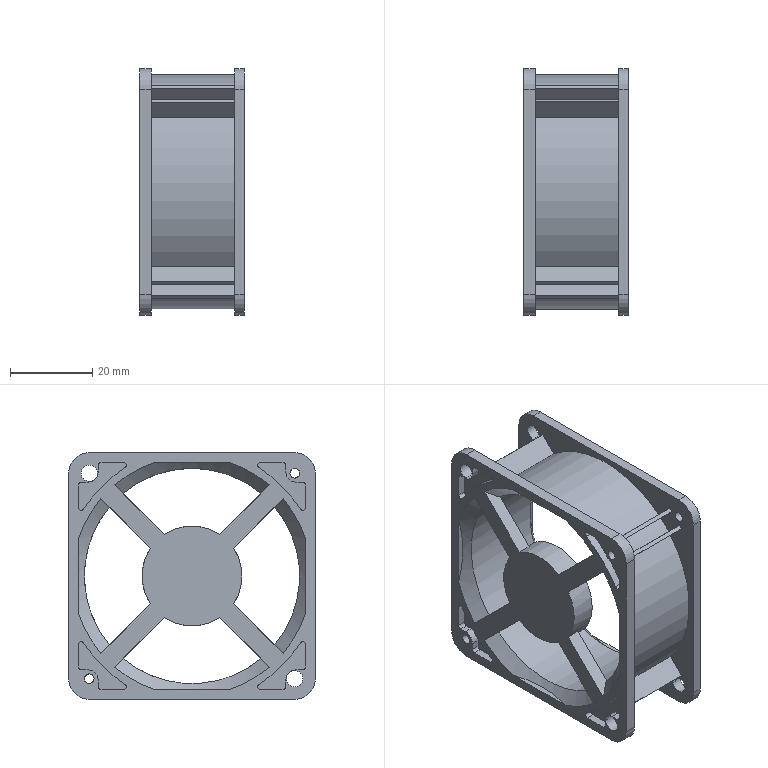Part | NX | features BREP 1 | 1 solid | 176 faces | box 25.5 x 60 x 60 mm | volume 18487 mm3 | plane 97 | cylinder 74 | cone 5 | commonest cylinder face diameters 1.429 x32 4.762 x8 10 x8 57.143 x8 61.905 x8 2.381 x4